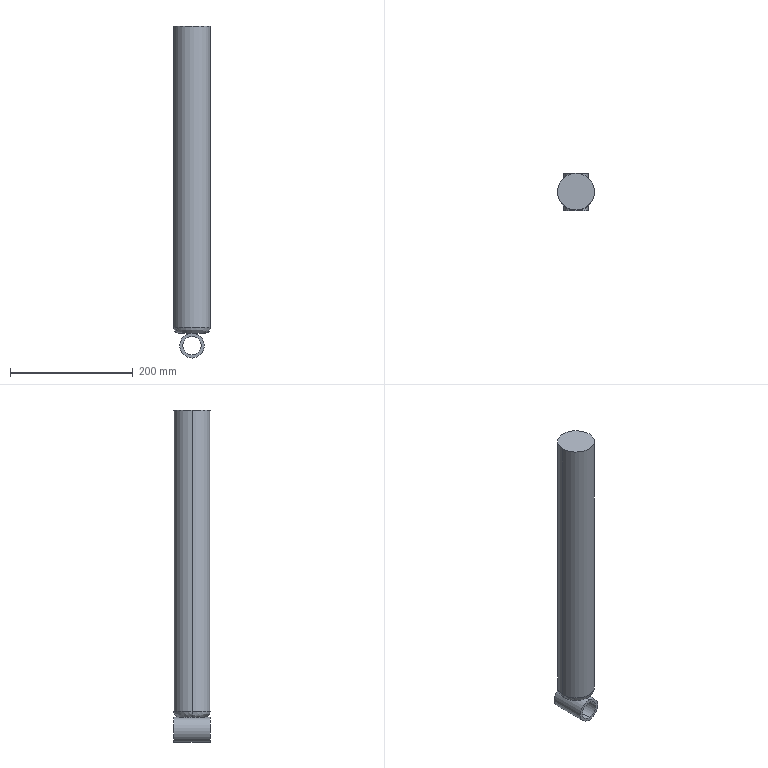Part | STEP file | Hydraulic cylinder A-400 | 2 solids | 12 faces | box 60 x 60 x 540 mm | volume 1442964 mm3 | cylinder 6 | plane 4 | spline 2 | commonest cylinder face diameters 30 x2 40 x2 60 x2
STEP:
#1=CARTESIAN_POINT('',(0.,-30.,0.));
#2=VERTEX_POINT('',#1);
#3=CARTESIAN_POINT('',(0.,-30.,-40.));
#4=VERTEX_POINT('',#3);
#5=CARTESIAN_POINT('',(0.,-30.,-20.));
#6=DIRECTION('',(0.,1.,0.));
#7=DIRECTION('',(0.,0.,1.));
#8=AXIS2_PLACEMENT_3D('',#5,#6,#7);
#9=CIRCLE('',#8,20.);
#10=EDGE_CURVE('',#2,#4,#9,.T.);
#11=ORIENTED_EDGE('',*,*,#10,.T.);
#12=CARTESIAN_POINT('',(0.,30.,-40.));
#13=VERTEX_POINT('',#12);
#14=CARTESIAN_POINT('',(0.,-30.,-40.));
#15=DIRECTION('',(0.,1.,0.));
#16=VECTOR('',#15,1000.);
#17=LINE('',#14,#16);
#18=EDGE_CURVE('',#4,#13,#17,.T.);
#19=ORIENTED_EDGE('',*,*,#18,.T.);
#20=CARTESIAN_POINT('',(0.,30.,0.));
#21=VERTEX_POINT('',#20);
#22=CARTESIAN_POINT('',(0.,30.,-20.));
#23=DIRECTION('',(0.,-1.,0.));
#24=DIRECTION('',(0.,0.,1.));
#25=AXIS2_PLACEMENT_3D('',#22,#23,#24);
#26=CIRCLE('',#25,20.);
#27=EDGE_CURVE('',#13,#21,#26,.T.);
#28=ORIENTED_EDGE('',*,*,#27,.T.);
#29=CARTESIAN_POINT('',(0.,-30.,0.));
#30=DIRECTION('',(0.,1.,0.));
#31=VECTOR('',#30,1000.);
#32=LINE('',#29,#31);
#33=EDGE_CURVE('',#2,#21,#32,.T.);
#34=ORIENTED_EDGE('',*,*,#33,.F.);
#35=EDGE_LOOP('',(#11,#19,#28,#34));
#36=FACE_OUTER_BOUND('',#35,.T.);
#37=CARTESIAN_POINT('',(0.,-30.,-20.));
#38=DIRECTION('',(0.,1.,0.));
#39=DIRECTION('',(0.,0.,1.));
#40=AXIS2_PLACEMENT_3D('',#37,#38,#39);
#41=CYLINDRICAL_SURFACE('',#40,20.);
#42=ADVANCED_FACE('',(#36),#41,.T.);
#43=CARTESIAN_POINT('',(0.,-30.,-5.));
#44=VERTEX_POINT('',#43);
#45=CARTESIAN_POINT('',(0.,-30.,-35.));
#46=VERTEX_POINT('',#45);
#47=CARTESIAN_POINT('',(0.,-30.,-20.));
#48=DIRECTION('',(0.,-1.,0.));
#49=DIRECTION('',(0.,0.,1.));
#50=AXIS2_PLACEMENT_3D('',#47,#48,#49);
#51=CIRCLE('',#50,15.);
#52=EDGE_CURVE('',#44,#46,#51,.T.);
#53=ORIENTED_EDGE('',*,*,#52,.T.);
#54=CARTESIAN_POINT('',(0.,30.,-35.));
#55=VERTEX_POINT('',#54);
#56=CARTESIAN_POINT('',(0.,-30.,-35.));
#57=DIRECTION('',(0.,1.,0.));
#58=VECTOR('',#57,1000.);
#59=LINE('',#56,#58);
#60=EDGE_CURVE('',#46,#55,#59,.T.);
#61=ORIENTED_EDGE('',*,*,#60,.T.);
#62=CARTESIAN_POINT('',(0.,30.,-5.));
#63=VERTEX_POINT('',#62);
#64=CARTESIAN_POINT('',(0.,30.,-20.));
#65=DIRECTION('',(0.,-1.,0.));
#66=DIRECTION('',(0.,0.,1.));
#67=AXIS2_PLACEMENT_3D('',#64,#65,#66);
#68=CIRCLE('',#67,15.);
#69=EDGE_CURVE('',#63,#55,#68,.T.);
#70=ORIENTED_EDGE('',*,*,#69,.F.);
#71=CARTESIAN_POINT('',(0.,-30.,-5.));
#72=DIRECTION('',(0.,1.,0.));
#73=VECTOR('',#72,1000.);
#74=LINE('',#71,#73);
#75=EDGE_CURVE('',#44,#63,#74,.T.);
#76=ORIENTED_EDGE('',*,*,#75,.F.);
#77=EDGE_LOOP('',(#53,#61,#70,#76));
#78=FACE_OUTER_BOUND('',#77,.T.);
#79=CARTESIAN_POINT('',(0.,-30.,-20.));
#80=DIRECTION('',(0.,1.,0.));
#81=DIRECTION('',(0.,0.,1.));
#82=AXIS2_PLACEMENT_3D('',#79,#80,#81);
#83=CYLINDRICAL_SURFACE('',#82,15.);
#84=ADVANCED_FACE('',(#78),#83,.F.);
#85=ORIENTED_EDGE('',*,*,#18,.F.);
#86=CARTESIAN_POINT('',(0.,-30.,-20.));
#87=DIRECTION('',(0.,1.,0.));
#88=DIRECTION('',(0.,0.,1.));
#89=AXIS2_PLACEMENT_3D('',#86,#87,#88);
#90=CIRCLE('',#89,20.);
#91=EDGE_CURVE('',#4,#2,#90,.T.);
#92=ORIENTED_EDGE('',*,*,#91,.T.);
#93=ORIENTED_EDGE('',*,*,#33,.T.);
#94=CARTESIAN_POINT('',(0.,30.,-20.));
#95=DIRECTION('',(0.,-1.,0.));
#96=DIRECTION('',(0.,0.,1.));
#97=AXIS2_PLACEMENT_3D('',#94,#95,#96);
#98=CIRCLE('',#97,20.);
#99=EDGE_CURVE('',#21,#13,#98,.T.);
#100=ORIENTED_EDGE('',*,*,#99,.T.);
#101=EDGE_LOOP('',(#85,#92,#93,#100));
#102=FACE_OUTER_BOUND('',#101,.T.);
#103=CARTESIAN_POINT('',(0.,-30.,-20.));
#104=DIRECTION('',(0.,1.,0.));
#105=DIRECTION('',(0.,0.,1.));
#106=AXIS2_PLACEMENT_3D('',#103,#104,#105);
#107=CYLINDRICAL_SURFACE('',#106,20.);
#108=ADVANCED_FACE('',(#102),#107,.T.);
#109=ORIENTED_EDGE('',*,*,#69,.T.);
#110=CARTESIAN_POINT('',(0.,30.,-20.));
#111=DIRECTION('',(0.,-1.,0.));
#112=DIRECTION('',(0.,0.,1.));
#113=AXIS2_PLACEMENT_3D('',#110,#111,#112);
#114=CIRCLE('',#113,15.);
#115=EDGE_CURVE('',#55,#63,#114,.T.);
#116=ORIENTED_EDGE('',*,*,#115,.T.);
#117=EDGE_LOOP('',(#109,#116));
#118=FACE_BOUND('',#117,.T.);
#119=ORIENTED_EDGE('',*,*,#99,.F.);
#120=ORIENTED_EDGE('',*,*,#27,.F.);
#121=EDGE_LOOP('',(#119,#120));
#122=FACE_OUTER_BOUND('',#121,.T.);
#123=CARTESIAN_POINT('',(0.,30.,-20.));
#124=DIRECTION('',(0.,1.,0.));
#125=DIRECTION('',(0.,0.,1.));
#126=AXIS2_PLACEMENT_3D('',#123,#124,#125);
#127=PLANE('',#126);
#128=ADVANCED_FACE('',(#118,#122),#127,.T.);
#129=ORIENTED_EDGE('',*,*,#10,.F.);
#130=ORIENTED_EDGE('',*,*,#91,.F.);
#131=EDGE_LOOP('',(#129,#130));
#132=FACE_OUTER_BOUND('',#131,.T.);
#133=ORIENTED_EDGE('',*,*,#52,.F.);
#134=CARTESIAN_POINT('',(0.,-30.,-20.));
#135=DIRECTION('',(0.,-1.,0.));
#136=DIRECTION('',(0.,0.,1.));
#137=AXIS2_PLACEMENT_3D('',#134,#135,#136);
#138=CIRCLE('',#137,15.);
#139=EDGE_CURVE('',#46,#44,#138,.T.);
#140=ORIENTED_EDGE('',*,*,#139,.F.);
#141=EDGE_LOOP('',(#133,#140));
#142=FACE_BOUND('',#141,.T.);
#143=CARTESIAN_POINT('',(0.,-30.,-20.));
#144=DIRECTION('',(0.,1.,0.));
#145=DIRECTION('',(0.,0.,1.));
#146=AXIS2_PLACEMENT_3D('',#143,#144,#145);
#147=PLANE('',#146);
#148=ADVANCED_FACE('',(#132,#142),#147,.F.);
#149=ORIENTED_EDGE('',*,*,#60,.F.);
#150=ORIENTED_EDGE('',*,*,#139,.T.);
#151=ORIENTED_EDGE('',*,*,#75,.T.);
#152=ORIENTED_EDGE('',*,*,#115,.F.);
#153=EDGE_LOOP('',(#149,#150,#151,#152));
#154=FACE_OUTER_BOUND('',#153,.T.);
#155=CARTESIAN_POINT('',(0.,-30.,-20.));
#156=DIRECTION('',(0.,1.,0.));
#157=DIRECTION('',(0.,0.,1.));
#158=AXIS2_PLACEMENT_3D('',#155,#156,#157);
#159=CYLINDRICAL_SURFACE('',#158,15.);
#160=ADVANCED_FACE('',(#154),#159,.F.);
#161=CLOSED_SHELL('',(#42,#84,#108,#128,#148,#160));
#162=MANIFOLD_SOLID_BREP('',#161);
#163=CARTESIAN_POINT('',(-30.,0.,10.));
#164=VERTEX_POINT('',#163);
#165=CARTESIAN_POINT('',(30.,0.,10.));
#166=VERTEX_POINT('',#165);
#167=CARTESIAN_POINT('',(0.,0.,10.));
#168=DIRECTION('',(0.,0.,1.));
#169=DIRECTION('',(-1.,0.,0.));
#170=AXIS2_PLACEMENT_3D('',#167,#168,#169);
#171=CIRCLE('',#170,30.);
#172=EDGE_CURVE('',#164,#166,#171,.T.);
#173=ORIENTED_EDGE('',*,*,#172,.F.);
#174=CARTESIAN_POINT('',(-20.,0.,0.));
#175=VERTEX_POINT('',#174);
#176=CARTESIAN_POINT('',(-20.,0.,10.));
#177=DIRECTION('',(0.,-1.,0.));
#178=DIRECTION('',(-1.,0.,0.));
#179=AXIS2_PLACEMENT_3D('',#176,#177,#178);
#180=CIRCLE('',#179,10.);
#181=EDGE_CURVE('',#164,#175,#180,.T.);
#182=ORIENTED_EDGE('',*,*,#181,.T.);
#183=CARTESIAN_POINT('',(20.,0.,0.));
#184=VERTEX_POINT('',#183);
#185=CARTESIAN_POINT('',(-20.,0.,0.));
#186=CARTESIAN_POINT('',(-20.,-40.,0.));
#187=CARTESIAN_POINT('',(20.,-40.,0.));
#188=CARTESIAN_POINT('',(20.,0.,0.));
#189=(BOUNDED_CURVE()B_SPLINE_CURVE(3,(#185,#186,#187,#188),.UNSPECIFIED.,.F.,.F.)B_SPLINE_CURVE_WITH_KNOTS((4,4),(0.,1.),.UNSPECIFIED.)CURVE()GEOMETRIC_REPRESENTATION_ITEM()RATIONAL_B_SPLINE_CURVE((1.,0.3333,0.3333,1.))REPRESENTATION_ITEM(''));
#190=EDGE_CURVE('',#175,#184,#189,.T.);
#191=ORIENTED_EDGE('',*,*,#190,.T.);
#192=CARTESIAN_POINT('',(20.,0.,10.));
#193=DIRECTION('',(0.,1.,0.));
#194=DIRECTION('',(1.,0.,0.));
#195=AXIS2_PLACEMENT_3D('',#192,#193,#194);
#196=CIRCLE('',#195,10.);
#197=EDGE_CURVE('',#166,#184,#196,.T.);
#198=ORIENTED_EDGE('',*,*,#197,.F.);
#199=EDGE_LOOP('',(#173,#182,#191,#198));
#200=FACE_OUTER_BOUND('',#199,.T.);
#201=CARTESIAN_POINT('',(-30.,0.,10.));
#202=CARTESIAN_POINT('',(-30.,-60.,10.));
#203=CARTESIAN_POINT('',(30.,-60.,10.));
#204=CARTESIAN_POINT('',(30.,0.,10.));
#205=CARTESIAN_POINT('',(-30.,0.,4.142));
#206=CARTESIAN_POINT('',(-30.,-60.,4.142));
#207=CARTESIAN_POINT('',(30.,-60.,4.142));
#208=CARTESIAN_POINT('',(30.,0.,4.142));
#209=CARTESIAN_POINT('',(-25.858,0.,0.));
#210=CARTESIAN_POINT('',(-25.858,-51.716,0.));
#211=CARTESIAN_POINT('',(25.858,-51.716,0.));
#212=CARTESIAN_POINT('',(25.858,0.,0.));
#213=CARTESIAN_POINT('',(-20.,0.,0.));
#214=CARTESIAN_POINT('',(-20.,-40.,0.));
#215=CARTESIAN_POINT('',(20.,-40.,0.));
#216=CARTESIAN_POINT('',(20.,0.,0.));
#217=(BOUNDED_SURFACE()B_SPLINE_SURFACE(3,3,((#201,#202,#203,#204),(#205,#206,#207,#208),(#209,#210,#211,#212),(#213,#214,#215,#216)),.UNSPECIFIED.,.F.,.F.,.F.)B_SPLINE_SURFACE_WITH_KNOTS((4,4),(4,4),(0.,1.),(0.,1.),.UNSPECIFIED.)GEOMETRIC_REPRESENTATION_ITEM()RATIONAL_B_SPLINE_SURFACE(((1.,0.3333,0.3333,1.),(0.8047,0.2682,0.2682,0.8047),(0.8047,0.2682,0.2682,0.8047),(1.,0.3333,0.3333,1.)))REPRESENTATION_ITEM('')SURFACE());
#218=ADVANCED_FACE('',(#200),#217,.T.);
#219=CARTESIAN_POINT('',(30.,0.,500.));
#220=VERTEX_POINT('',#219);
#221=CARTESIAN_POINT('',(-30.,0.,500.));
#222=VERTEX_POINT('',#221);
#223=CARTESIAN_POINT('',(0.,0.,500.));
#224=DIRECTION('',(0.,0.,1.));
#225=DIRECTION('',(1.,0.,0.));
#226=AXIS2_PLACEMENT_3D('',#223,#224,#225);
#227=CIRCLE('',#226,30.);
#228=EDGE_CURVE('',#220,#222,#227,.T.);
#229=ORIENTED_EDGE('',*,*,#228,.F.);
#230=CARTESIAN_POINT('',(30.,0.,350.));
#231=DIRECTION('',(0.,0.,-1.));
#232=VECTOR('',#231,1000.);
#233=LINE('',#230,#232);
#234=EDGE_CURVE('',#220,#166,#233,.T.);
#235=ORIENTED_EDGE('',*,*,#234,.T.);
#236=CARTESIAN_POINT('',(0.,0.,10.));
#237=DIRECTION('',(0.,0.,1.));
#238=DIRECTION('',(-1.,0.,0.));
#239=AXIS2_PLACEMENT_3D('',#236,#237,#238);
#240=CIRCLE('',#239,30.);
#241=EDGE_CURVE('',#166,#164,#240,.T.);
#242=ORIENTED_EDGE('',*,*,#241,.T.);
#243=CARTESIAN_POINT('',(-30.,0.,350.));
#244=DIRECTION('',(0.,0.,-1.));
#245=VECTOR('',#244,1000.);
#246=LINE('',#243,#245);
#247=EDGE_CURVE('',#222,#164,#246,.T.);
#248=ORIENTED_EDGE('',*,*,#247,.F.);
#249=EDGE_LOOP('',(#229,#235,#242,#248));
#250=FACE_OUTER_BOUND('',#249,.T.);
#251=CARTESIAN_POINT('',(0.,0.,350.));
#252=DIRECTION('',(0.,0.,-1.));
#253=DIRECTION('',(-1.,0.,0.));
#254=AXIS2_PLACEMENT_3D('',#251,#252,#253);
#255=CYLINDRICAL_SURFACE('',#254,30.);
#256=ADVANCED_FACE('',(#250),#255,.T.);
#257=ORIENTED_EDGE('',*,*,#234,.F.);
#258=CARTESIAN_POINT('',(0.,0.,500.));
#259=DIRECTION('',(0.,0.,1.));
#260=DIRECTION('',(1.,0.,0.));
#261=AXIS2_PLACEMENT_3D('',#258,#259,#260);
#262=CIRCLE('',#261,30.);
#263=EDGE_CURVE('',#222,#220,#262,.T.);
#264=ORIENTED_EDGE('',*,*,#263,.F.);
#265=ORIENTED_EDGE('',*,*,#247,.T.);
#266=ORIENTED_EDGE('',*,*,#172,.T.);
#267=EDGE_LOOP('',(#257,#264,#265,#266));
#268=FACE_OUTER_BOUND('',#267,.T.);
#269=CARTESIAN_POINT('',(0.,0.,350.));
#270=DIRECTION('',(0.,0.,-1.));
#271=DIRECTION('',(-1.,0.,0.));
#272=AXIS2_PLACEMENT_3D('',#269,#270,#271);
#273=CYLINDRICAL_SURFACE('',#272,30.);
#274=ADVANCED_FACE('',(#268),#273,.T.);
#275=ORIENTED_EDGE('',*,*,#181,.F.);
#276=ORIENTED_EDGE('',*,*,#241,.F.);
#277=ORIENTED_EDGE('',*,*,#197,.T.);
#278=CARTESIAN_POINT('',(20.,0.,0.));
#279=CARTESIAN_POINT('',(20.,40.,0.));
#280=CARTESIAN_POINT('',(-20.,40.,0.));
#281=CARTESIAN_POINT('',(-20.,0.,0.));
#282=(BOUNDED_CURVE()B_SPLINE_CURVE(3,(#278,#279,#280,#281),.UNSPECIFIED.,.F.,.F.)B_SPLINE_CURVE_WITH_KNOTS((4,4),(0.,1.),.UNSPECIFIED.)CURVE()GEOMETRIC_REPRESENTATION_ITEM()RATIONAL_B_SPLINE_CURVE((1.,0.3333,0.3333,1.))REPRESENTATION_ITEM(''));
#283=EDGE_CURVE('',#184,#175,#282,.T.);
#284=ORIENTED_EDGE('',*,*,#283,.T.);
#285=EDGE_LOOP('',(#275,#276,#277,#284));
#286=FACE_OUTER_BOUND('',#285,.T.);
#287=CARTESIAN_POINT('',(30.,0.,10.));
#288=CARTESIAN_POINT('',(30.,60.,10.));
#289=CARTESIAN_POINT('',(-30.,60.,10.));
#290=CARTESIAN_POINT('',(-30.,0.,10.));
#291=CARTESIAN_POINT('',(30.,0.,4.142));
#292=CARTESIAN_POINT('',(30.,60.,4.142));
#293=CARTESIAN_POINT('',(-30.,60.,4.142));
#294=CARTESIAN_POINT('',(-30.,0.,4.142));
#295=CARTESIAN_POINT('',(25.858,0.,0.));
#296=CARTESIAN_POINT('',(25.858,51.716,0.));
#297=CARTESIAN_POINT('',(-25.858,51.716,0.));
#298=CARTESIAN_POINT('',(-25.858,0.,0.));
#299=CARTESIAN_POINT('',(20.,0.,0.));
#300=CARTESIAN_POINT('',(20.,40.,0.));
#301=CARTESIAN_POINT('',(-20.,40.,0.));
#302=CARTESIAN_POINT('',(-20.,0.,0.));
#303=(BOUNDED_SURFACE()B_SPLINE_SURFACE(3,3,((#287,#288,#289,#290),(#291,#292,#293,#294),(#295,#296,#297,#298),(#299,#300,#301,#302)),.UNSPECIFIED.,.F.,.F.,.F.)B_SPLINE_SURFACE_WITH_KNOTS((4,4),(4,4),(0.,1.),(0.,1.),.UNSPECIFIED.)GEOMETRIC_REPRESENTATION_ITEM()RATIONAL_B_SPLINE_SURFACE(((1.,0.3333,0.3333,1.),(0.8047,0.2682,0.2682,0.8047),(0.8047,0.2682,0.2682,0.8047),(1.,0.3333,0.3333,1.)))REPRESENTATION_ITEM('')SURFACE());
#304=ADVANCED_FACE('',(#286),#303,.T.);
#305=ORIENTED_EDGE('',*,*,#283,.F.);
#306=ORIENTED_EDGE('',*,*,#190,.F.);
#307=EDGE_LOOP('',(#305,#306));
#308=FACE_OUTER_BOUND('',#307,.T.);
#309=CARTESIAN_POINT('',(0.,0.,0.));
#310=DIRECTION('',(0.,0.,1.));
#311=DIRECTION('',(1.,0.,0.));
#312=AXIS2_PLACEMENT_3D('',#309,#310,#311);
#313=PLANE('',#312);
#314=ADVANCED_FACE('',(#308),#313,.F.);
#315=ORIENTED_EDGE('',*,*,#263,.T.);
#316=ORIENTED_EDGE('',*,*,#228,.T.);
#317=EDGE_LOOP('',(#315,#316));
#318=FACE_OUTER_BOUND('',#317,.T.);
#319=CARTESIAN_POINT('',(0.,0.,500.));
#320=DIRECTION('',(0.,0.,1.));
#321=DIRECTION('',(1.,0.,0.));
#322=AXIS2_PLACEMENT_3D('',#319,#320,#321);
#323=PLANE('',#322);
#324=ADVANCED_FACE('',(#318),#323,.T.);
#325=CLOSED_SHELL('',(#218,#256,#274,#304,#314,#324));
#326=MANIFOLD_SOLID_BREP('',#325);
#327=CARTESIAN_POINT('',(0.,0.,0.));
#328=DIRECTION('',(0.,0.,1.));
#329=DIRECTION('',(1.,0.,0.));
#330=AXIS2_PLACEMENT_3D('',#327,#328,#329);
#331=(LENGTH_UNIT()NAMED_UNIT(*)SI_UNIT(.MILLI.,.METRE.));
#332=UNCERTAINTY_MEASURE_WITH_UNIT(LENGTH_MEASURE(0.00001),#331,'','');
#333=(NAMED_UNIT(*)PLANE_ANGLE_UNIT()SI_UNIT($,.RADIAN.));
#334=(NAMED_UNIT(*)SI_UNIT($,.STERADIAN.)SOLID_ANGLE_UNIT());
#335=(GEOMETRIC_REPRESENTATION_CONTEXT(3)GLOBAL_UNCERTAINTY_ASSIGNED_CONTEXT((#332))GLOBAL_UNIT_ASSIGNED_CONTEXT((#331,#333,#334))REPRESENTATION_CONTEXT('',''));
#336=ADVANCED_BREP_SHAPE_REPRESENTATION('',(#162,#326,#330),#335);